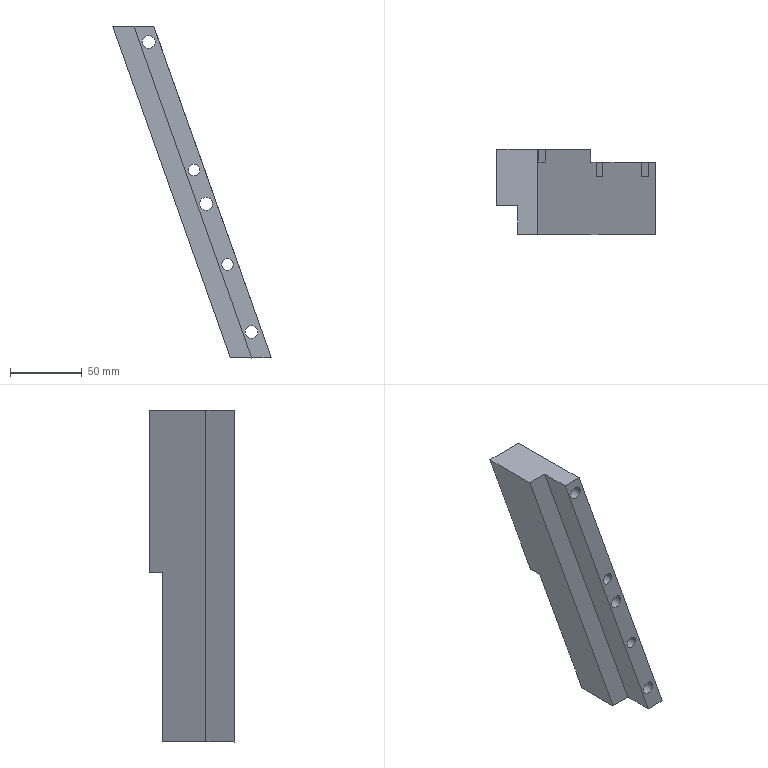Part | STEP file | SLIDE1-PLATE_id550_x_t | 1 solid | 27 faces | box 110.798 x 59.5 x 232 mm | volume 275836 mm3 | plane 19 | cylinder 8 | commonest cylinder face diameters 9 x3 14 x3 8 x2
STEP:
#1=CARTESIAN_POINT('',(86.433,-9.5,-60.698));
#2=VERTEX_POINT('',#1);
#3=CARTESIAN_POINT('',(81.759,-9.5,-47.502));
#4=VERTEX_POINT('',#3);
#5=CARTESIAN_POINT('',(84.096,-9.5,-54.1));
#6=DIRECTION('',(0.,1.,0.));
#7=DIRECTION('',(0.,0.,1.));
#8=AXIS2_PLACEMENT_3D('',#5,#6,#7);
#9=CIRCLE('',#8,7.);
#10=EDGE_CURVE('',#2,#4,#9,.T.);
#11=ORIENTED_EDGE('',*,*,#10,.F.);
#12=CARTESIAN_POINT('',(86.433,-0.5,-60.698));
#13=VERTEX_POINT('',#12);
#14=CARTESIAN_POINT('',(86.433,-0.5,-60.698));
#15=DIRECTION('',(0.,1.,0.));
#16=VECTOR('',#15,1.);
#17=LINE('',#14,#16);
#18=EDGE_CURVE('',#2,#13,#17,.T.);
#19=ORIENTED_EDGE('',*,*,#18,.T.);
#20=CARTESIAN_POINT('',(81.759,-0.5,-47.502));
#21=VERTEX_POINT('',#20);
#22=CARTESIAN_POINT('',(84.096,-0.5,-54.1));
#23=DIRECTION('',(0.,-1.,0.));
#24=DIRECTION('',(0.,0.,1.));
#25=AXIS2_PLACEMENT_3D('',#22,#23,#24);
#26=CIRCLE('',#25,7.);
#27=EDGE_CURVE('',#21,#13,#26,.T.);
#28=ORIENTED_EDGE('',*,*,#27,.F.);
#29=CARTESIAN_POINT('',(81.759,-0.5,-47.502));
#30=DIRECTION('',(0.,-1.,0.));
#31=VECTOR('',#30,1.);
#32=LINE('',#29,#31);
#33=EDGE_CURVE('',#21,#4,#32,.T.);
#34=ORIENTED_EDGE('',*,*,#33,.T.);
#35=EDGE_LOOP('',(#11,#19,#28,#34));
#36=FACE_OUTER_BOUND('',#35,.T.);
#37=CARTESIAN_POINT('',(84.096,-0.5,-54.1));
#38=DIRECTION('',(0.,1.,0.));
#39=DIRECTION('',(0.,0.,1.));
#40=AXIS2_PLACEMENT_3D('',#37,#38,#39);
#41=CYLINDRICAL_SURFACE('',#40,7.);
#42=ADVANCED_FACE('',(#36),#41,.F.);
#43=CARTESIAN_POINT('',(84.096,-60.,-49.6));
#44=VERTEX_POINT('',#43);
#45=CARTESIAN_POINT('',(84.096,-60.,-54.1));
#46=DIRECTION('',(0.,1.,0.));
#47=DIRECTION('',(0.,0.,1.));
#48=AXIS2_PLACEMENT_3D('',#45,#46,#47);
#49=CIRCLE('',#48,4.5);
#50=EDGE_CURVE('',#44,#44,#49,.T.);
#51=ORIENTED_EDGE('',*,*,#50,.F.);
#52=EDGE_LOOP('',(#51));
#53=FACE_BOUND('',#52,.T.);
#54=CARTESIAN_POINT('',(84.096,-9.5,-49.6));
#55=VERTEX_POINT('',#54);
#56=CARTESIAN_POINT('',(84.096,-9.5,-54.1));
#57=DIRECTION('',(0.,-1.,0.));
#58=DIRECTION('',(0.,0.,1.));
#59=AXIS2_PLACEMENT_3D('',#56,#57,#58);
#60=CIRCLE('',#59,4.5);
#61=EDGE_CURVE('',#55,#55,#60,.T.);
#62=ORIENTED_EDGE('',*,*,#61,.F.);
#63=EDGE_LOOP('',(#62));
#64=FACE_BOUND('',#63,.T.);
#65=CARTESIAN_POINT('',(84.096,-0.5,-54.1));
#66=DIRECTION('',(0.,1.,0.));
#67=DIRECTION('',(0.,0.,1.));
#68=AXIS2_PLACEMENT_3D('',#65,#66,#67);
#69=CYLINDRICAL_SURFACE('',#68,4.5);
#70=ADVANCED_FACE('',(#53,#64),#69,.F.);
#71=CARTESIAN_POINT('',(115.807,-60.,-139.65));
#72=VERTEX_POINT('',#71);
#73=CARTESIAN_POINT('',(115.807,-60.,-143.65));
#74=DIRECTION('',(0.,1.,0.));
#75=DIRECTION('',(0.,0.,1.));
#76=AXIS2_PLACEMENT_3D('',#73,#74,#75);
#77=CIRCLE('',#76,4.);
#78=EDGE_CURVE('',#72,#72,#77,.T.);
#79=ORIENTED_EDGE('',*,*,#78,.F.);
#80=EDGE_LOOP('',(#79));
#81=FACE_BOUND('',#80,.T.);
#82=CARTESIAN_POINT('',(115.807,-0.5,-139.65));
#83=VERTEX_POINT('',#82);
#84=CARTESIAN_POINT('',(115.807,-0.5,-143.65));
#85=DIRECTION('',(0.,-1.,0.));
#86=DIRECTION('',(0.,0.,1.));
#87=AXIS2_PLACEMENT_3D('',#84,#85,#86);
#88=CIRCLE('',#87,4.);
#89=EDGE_CURVE('',#83,#83,#88,.T.);
#90=ORIENTED_EDGE('',*,*,#89,.F.);
#91=EDGE_LOOP('',(#90));
#92=FACE_BOUND('',#91,.T.);
#93=CARTESIAN_POINT('',(115.807,-0.5,-143.65));
#94=DIRECTION('',(0.,1.,0.));
#95=DIRECTION('',(0.,0.,1.));
#96=AXIS2_PLACEMENT_3D('',#93,#94,#95);
#97=CYLINDRICAL_SURFACE('',#96,4.);
#98=ADVANCED_FACE('',(#81,#92),#97,.F.);
#99=CARTESIAN_POINT('',(124.15,-60.,-162.71));
#100=VERTEX_POINT('',#99);
#101=CARTESIAN_POINT('',(124.15,-60.,-167.21));
#102=DIRECTION('',(0.,1.,0.));
#103=DIRECTION('',(0.,0.,1.));
#104=AXIS2_PLACEMENT_3D('',#101,#102,#103);
#105=CIRCLE('',#104,4.5);
#106=EDGE_CURVE('',#100,#100,#105,.T.);
#107=ORIENTED_EDGE('',*,*,#106,.F.);
#108=EDGE_LOOP('',(#107));
#109=FACE_BOUND('',#108,.T.);
#110=CARTESIAN_POINT('',(124.15,-19.5,-162.71));
#111=VERTEX_POINT('',#110);
#112=CARTESIAN_POINT('',(124.15,-19.5,-167.21));
#113=DIRECTION('',(0.,-1.,0.));
#114=DIRECTION('',(0.,0.,1.));
#115=AXIS2_PLACEMENT_3D('',#112,#113,#114);
#116=CIRCLE('',#115,4.5);
#117=EDGE_CURVE('',#111,#111,#116,.T.);
#118=ORIENTED_EDGE('',*,*,#117,.F.);
#119=EDGE_LOOP('',(#118));
#120=FACE_BOUND('',#119,.T.);
#121=CARTESIAN_POINT('',(124.15,-0.5,-167.21));
#122=DIRECTION('',(0.,1.,0.));
#123=DIRECTION('',(0.,0.,1.));
#124=AXIS2_PLACEMENT_3D('',#121,#122,#123);
#125=CYLINDRICAL_SURFACE('',#124,4.5);
#126=ADVANCED_FACE('',(#109,#120),#125,.F.);
#127=CARTESIAN_POINT('',(155.862,-60.,-252.26));
#128=VERTEX_POINT('',#127);
#129=CARTESIAN_POINT('',(155.862,-60.,-256.76));
#130=DIRECTION('',(0.,1.,0.));
#131=DIRECTION('',(0.,0.,1.));
#132=AXIS2_PLACEMENT_3D('',#129,#130,#131);
#133=CIRCLE('',#132,4.5);
#134=EDGE_CURVE('',#128,#128,#133,.T.);
#135=ORIENTED_EDGE('',*,*,#134,.F.);
#136=EDGE_LOOP('',(#135));
#137=FACE_BOUND('',#136,.T.);
#138=CARTESIAN_POINT('',(155.862,-19.5,-252.26));
#139=VERTEX_POINT('',#138);
#140=CARTESIAN_POINT('',(155.862,-19.5,-256.76));
#141=DIRECTION('',(0.,-1.,0.));
#142=DIRECTION('',(0.,0.,1.));
#143=AXIS2_PLACEMENT_3D('',#140,#141,#142);
#144=CIRCLE('',#143,4.5);
#145=EDGE_CURVE('',#139,#139,#144,.T.);
#146=ORIENTED_EDGE('',*,*,#145,.F.);
#147=EDGE_LOOP('',(#146));
#148=FACE_BOUND('',#147,.T.);
#149=CARTESIAN_POINT('',(155.862,-0.5,-256.76));
#150=DIRECTION('',(0.,1.,0.));
#151=DIRECTION('',(0.,0.,1.));
#152=AXIS2_PLACEMENT_3D('',#149,#150,#151);
#153=CYLINDRICAL_SURFACE('',#152,4.5);
#154=ADVANCED_FACE('',(#137,#148),#153,.F.);
#155=CARTESIAN_POINT('',(155.956,-40.,-275.));
#156=VERTEX_POINT('',#155);
#157=CARTESIAN_POINT('',(73.8,-40.,-43.));
#158=VERTEX_POINT('',#157);
#159=CARTESIAN_POINT('',(63.323,-40.,-13.414));
#160=DIRECTION('',(-0.3338,0.,0.9426));
#161=VECTOR('',#160,1.);
#162=LINE('',#159,#161);
#163=EDGE_CURVE('',#156,#158,#162,.T.);
#164=ORIENTED_EDGE('',*,*,#163,.T.);
#165=CARTESIAN_POINT('',(58.948,-40.,-43.));
#166=VERTEX_POINT('',#165);
#167=CARTESIAN_POINT('',(83.348,-40.,-43.));
#168=DIRECTION('',(-1.,0.,0.));
#169=VECTOR('',#168,1.);
#170=LINE('',#167,#169);
#171=EDGE_CURVE('',#158,#166,#170,.T.);
#172=ORIENTED_EDGE('',*,*,#171,.T.);
#173=CARTESIAN_POINT('',(141.104,-40.,-275.));
#174=VERTEX_POINT('',#173);
#175=CARTESIAN_POINT('',(50.126,-40.,-18.087));
#176=DIRECTION('',(-0.3338,0.,0.9426));
#177=VECTOR('',#176,1.);
#178=LINE('',#175,#177);
#179=EDGE_CURVE('',#174,#166,#178,.T.);
#180=ORIENTED_EDGE('',*,*,#179,.F.);
#181=CARTESIAN_POINT('',(141.104,-40.,-275.));
#182=DIRECTION('',(1.,0.,0.));
#183=VECTOR('',#182,1.);
#184=LINE('',#181,#183);
#185=EDGE_CURVE('',#174,#156,#184,.T.);
#186=ORIENTED_EDGE('',*,*,#185,.T.);
#187=EDGE_LOOP('',(#164,#172,#180,#186));
#188=FACE_OUTER_BOUND('',#187,.T.);
#189=CARTESIAN_POINT('',(63.323,-40.,-13.414));
#190=DIRECTION('',(0.,1.,0.));
#191=DIRECTION('',(0.,0.,1.));
#192=AXIS2_PLACEMENT_3D('',#189,#190,#191);
#193=PLANE('',#192);
#194=ADVANCED_FACE('',(#188),#193,.F.);
#195=ORIENTED_EDGE('',*,*,#163,.F.);
#196=CARTESIAN_POINT('',(155.956,-60.,-275.));
#197=VERTEX_POINT('',#196);
#198=CARTESIAN_POINT('',(155.956,-0.5,-275.));
#199=DIRECTION('',(0.,-1.,0.));
#200=VECTOR('',#199,1.);
#201=LINE('',#198,#200);
#202=EDGE_CURVE('',#156,#197,#201,.T.);
#203=ORIENTED_EDGE('',*,*,#202,.T.);
#204=CARTESIAN_POINT('',(73.8,-60.,-43.));
#205=VERTEX_POINT('',#204);
#206=CARTESIAN_POINT('',(73.8,-60.,-43.));
#207=DIRECTION('',(0.3338,0.,-0.9426));
#208=VECTOR('',#207,1.);
#209=LINE('',#206,#208);
#210=EDGE_CURVE('',#205,#197,#209,.T.);
#211=ORIENTED_EDGE('',*,*,#210,.F.);
#212=CARTESIAN_POINT('',(73.8,-0.5,-43.));
#213=DIRECTION('',(0.,1.,0.));
#214=VECTOR('',#213,1.);
#215=LINE('',#212,#214);
#216=EDGE_CURVE('',#205,#158,#215,.T.);
#217=ORIENTED_EDGE('',*,*,#216,.T.);
#218=EDGE_LOOP('',(#195,#203,#211,#217));
#219=FACE_OUTER_BOUND('',#218,.T.);
#220=CARTESIAN_POINT('',(63.323,-60.,-13.414));
#221=DIRECTION('',(0.9426,0.,0.3338));
#222=DIRECTION('',(0.3338,0.,-0.9426));
#223=AXIS2_PLACEMENT_3D('',#220,#221,#222);
#224=PLANE('',#223);
#225=ADVANCED_FACE('',(#219),#224,.F.);
#226=CARTESIAN_POINT('',(126.487,-19.5,-173.808));
#227=VERTEX_POINT('',#226);
#228=CARTESIAN_POINT('',(121.814,-19.5,-160.612));
#229=VERTEX_POINT('',#228);
#230=CARTESIAN_POINT('',(124.15,-19.5,-167.21));
#231=DIRECTION('',(0.,1.,0.));
#232=DIRECTION('',(0.,0.,1.));
#233=AXIS2_PLACEMENT_3D('',#230,#231,#232);
#234=CIRCLE('',#233,7.);
#235=EDGE_CURVE('',#227,#229,#234,.T.);
#236=ORIENTED_EDGE('',*,*,#235,.F.);
#237=CARTESIAN_POINT('',(126.487,-9.5,-173.808));
#238=VERTEX_POINT('',#237);
#239=CARTESIAN_POINT('',(126.487,-0.5,-173.808));
#240=DIRECTION('',(0.,1.,0.));
#241=VECTOR('',#240,1.);
#242=LINE('',#239,#241);
#243=EDGE_CURVE('',#227,#238,#242,.T.);
#244=ORIENTED_EDGE('',*,*,#243,.T.);
#245=CARTESIAN_POINT('',(121.814,-9.5,-160.612));
#246=VERTEX_POINT('',#245);
#247=CARTESIAN_POINT('',(124.15,-9.5,-167.21));
#248=DIRECTION('',(0.,-1.,0.));
#249=DIRECTION('',(0.,0.,1.));
#250=AXIS2_PLACEMENT_3D('',#247,#248,#249);
#251=CIRCLE('',#250,7.);
#252=EDGE_CURVE('',#246,#238,#251,.T.);
#253=ORIENTED_EDGE('',*,*,#252,.F.);
#254=CARTESIAN_POINT('',(121.814,-0.5,-160.612));
#255=DIRECTION('',(0.,-1.,0.));
#256=VECTOR('',#255,1.);
#257=LINE('',#254,#256);
#258=EDGE_CURVE('',#246,#229,#257,.T.);
#259=ORIENTED_EDGE('',*,*,#258,.T.);
#260=EDGE_LOOP('',(#236,#244,#253,#259));
#261=FACE_OUTER_BOUND('',#260,.T.);
#262=CARTESIAN_POINT('',(124.15,-0.5,-167.21));
#263=DIRECTION('',(0.,1.,0.));
#264=DIRECTION('',(0.,0.,1.));
#265=AXIS2_PLACEMENT_3D('',#262,#263,#264);
#266=CYLINDRICAL_SURFACE('',#265,7.);
#267=ADVANCED_FACE('',(#261),#266,.F.);
#268=CARTESIAN_POINT('',(158.198,-19.5,-263.358));
#269=VERTEX_POINT('',#268);
#270=CARTESIAN_POINT('',(153.525,-19.5,-250.162));
#271=VERTEX_POINT('',#270);
#272=CARTESIAN_POINT('',(155.862,-19.5,-256.76));
#273=DIRECTION('',(0.,1.,0.));
#274=DIRECTION('',(0.,0.,1.));
#275=AXIS2_PLACEMENT_3D('',#272,#273,#274);
#276=CIRCLE('',#275,7.);
#277=EDGE_CURVE('',#269,#271,#276,.T.);
#278=ORIENTED_EDGE('',*,*,#277,.F.);
#279=CARTESIAN_POINT('',(158.198,-9.5,-263.358));
#280=VERTEX_POINT('',#279);
#281=CARTESIAN_POINT('',(158.198,-0.5,-263.358));
#282=DIRECTION('',(0.,1.,0.));
#283=VECTOR('',#282,1.);
#284=LINE('',#281,#283);
#285=EDGE_CURVE('',#269,#280,#284,.T.);
#286=ORIENTED_EDGE('',*,*,#285,.T.);
#287=CARTESIAN_POINT('',(153.525,-9.5,-250.162));
#288=VERTEX_POINT('',#287);
#289=CARTESIAN_POINT('',(155.862,-9.5,-256.76));
#290=DIRECTION('',(0.,-1.,0.));
#291=DIRECTION('',(0.,0.,1.));
#292=AXIS2_PLACEMENT_3D('',#289,#290,#291);
#293=CIRCLE('',#292,7.);
#294=EDGE_CURVE('',#288,#280,#293,.T.);
#295=ORIENTED_EDGE('',*,*,#294,.F.);
#296=CARTESIAN_POINT('',(153.525,-0.5,-250.162));
#297=DIRECTION('',(0.,-1.,0.));
#298=VECTOR('',#297,1.);
#299=LINE('',#296,#298);
#300=EDGE_CURVE('',#288,#271,#299,.T.);
#301=ORIENTED_EDGE('',*,*,#300,.T.);
#302=EDGE_LOOP('',(#278,#286,#295,#301));
#303=FACE_OUTER_BOUND('',#302,.T.);
#304=CARTESIAN_POINT('',(155.862,-0.5,-256.76));
#305=DIRECTION('',(0.,1.,0.));
#306=DIRECTION('',(0.,0.,1.));
#307=AXIS2_PLACEMENT_3D('',#304,#305,#306);
#308=CYLINDRICAL_SURFACE('',#307,7.);
#309=ADVANCED_FACE('',(#303),#308,.F.);
#310=CARTESIAN_POINT('',(99.196,-0.5,-156.656));
#311=VERTEX_POINT('',#310);
#312=CARTESIAN_POINT('',(99.196,-9.5,-156.656));
#313=VERTEX_POINT('',#312);
#314=CARTESIAN_POINT('',(99.196,-0.5,-156.656));
#315=DIRECTION('',(0.,-1.,0.));
#316=VECTOR('',#315,1.);
#317=LINE('',#314,#316);
#318=EDGE_CURVE('',#311,#313,#317,.T.);
#319=ORIENTED_EDGE('',*,*,#318,.T.);
#320=CARTESIAN_POINT('',(141.104,-9.5,-275.));
#321=VERTEX_POINT('',#320);
#322=CARTESIAN_POINT('',(141.104,-9.5,-275.));
#323=DIRECTION('',(-0.3338,0.,0.9426));
#324=VECTOR('',#323,1.);
#325=LINE('',#322,#324);
#326=EDGE_CURVE('',#321,#313,#325,.T.);
#327=ORIENTED_EDGE('',*,*,#326,.F.);
#328=CARTESIAN_POINT('',(141.104,-0.5,-275.));
#329=DIRECTION('',(0.,-1.,0.));
#330=VECTOR('',#329,1.);
#331=LINE('',#328,#330);
#332=EDGE_CURVE('',#321,#174,#331,.T.);
#333=ORIENTED_EDGE('',*,*,#332,.T.);
#334=ORIENTED_EDGE('',*,*,#179,.T.);
#335=CARTESIAN_POINT('',(58.948,-0.5,-43.));
#336=VERTEX_POINT('',#335);
#337=CARTESIAN_POINT('',(58.948,-0.5,-43.));
#338=DIRECTION('',(0.,1.,0.));
#339=VECTOR('',#338,1.);
#340=LINE('',#337,#339);
#341=EDGE_CURVE('',#166,#336,#340,.T.);
#342=ORIENTED_EDGE('',*,*,#341,.T.);
#343=CARTESIAN_POINT('',(99.196,-0.5,-156.656));
#344=DIRECTION('',(-0.3338,0.,0.9426));
#345=VECTOR('',#344,1.);
#346=LINE('',#343,#345);
#347=EDGE_CURVE('',#311,#336,#346,.T.);
#348=ORIENTED_EDGE('',*,*,#347,.F.);
#349=EDGE_LOOP('',(#319,#327,#333,#334,#342,#348));
#350=FACE_OUTER_BOUND('',#349,.T.);
#351=CARTESIAN_POINT('',(50.126,-50.,-18.087));
#352=DIRECTION('',(-0.9426,0.,-0.3338));
#353=DIRECTION('',(-0.3338,0.,0.9426));
#354=AXIS2_PLACEMENT_3D('',#351,#352,#353);
#355=PLANE('',#354);
#356=ADVANCED_FACE('',(#350),#355,.T.);
#357=CARTESIAN_POINT('',(139.172,-60.,-205.63));
#358=VERTEX_POINT('',#357);
#359=CARTESIAN_POINT('',(139.172,-60.,-209.63));
#360=DIRECTION('',(0.,1.,0.));
#361=DIRECTION('',(0.,0.,1.));
#362=AXIS2_PLACEMENT_3D('',#359,#360,#361);
#363=CIRCLE('',#362,4.);
#364=EDGE_CURVE('',#358,#358,#363,.T.);
#365=ORIENTED_EDGE('',*,*,#364,.F.);
#366=EDGE_LOOP('',(#365));
#367=FACE_BOUND('',#366,.T.);
#368=CARTESIAN_POINT('',(139.172,-9.5,-205.63));
#369=VERTEX_POINT('',#368);
#370=CARTESIAN_POINT('',(139.172,-9.5,-209.63));
#371=DIRECTION('',(0.,-1.,0.));
#372=DIRECTION('',(0.,0.,1.));
#373=AXIS2_PLACEMENT_3D('',#370,#371,#372);
#374=CIRCLE('',#373,4.);
#375=EDGE_CURVE('',#369,#369,#374,.T.);
#376=ORIENTED_EDGE('',*,*,#375,.F.);
#377=EDGE_LOOP('',(#376));
#378=FACE_BOUND('',#377,.T.);
#379=CARTESIAN_POINT('',(139.172,-0.5,-209.63));
#380=DIRECTION('',(0.,1.,0.));
#381=DIRECTION('',(0.,0.,1.));
#382=AXIS2_PLACEMENT_3D('',#379,#380,#381);
#383=CYLINDRICAL_SURFACE('',#382,4.);
#384=ADVANCED_FACE('',(#367,#378),#383,.F.);
#385=CARTESIAN_POINT('',(164.797,-19.5,-261.022));
#386=VERTEX_POINT('',#385);
#387=CARTESIAN_POINT('',(164.797,-19.5,-261.022));
#388=DIRECTION('',(-0.9426,0.,-0.3338));
#389=VECTOR('',#388,1.);
#390=LINE('',#387,#389);
#391=EDGE_CURVE('',#386,#269,#390,.T.);
#392=ORIENTED_EDGE('',*,*,#391,.F.);
#393=CARTESIAN_POINT('',(164.797,-9.5,-261.022));
#394=VERTEX_POINT('',#393);
#395=CARTESIAN_POINT('',(164.797,-0.5,-261.022));
#396=DIRECTION('',(0.,-1.,0.));
#397=VECTOR('',#396,1.);
#398=LINE('',#395,#397);
#399=EDGE_CURVE('',#394,#386,#398,.T.);
#400=ORIENTED_EDGE('',*,*,#399,.F.);
#401=CARTESIAN_POINT('',(158.198,-9.5,-263.358));
#402=DIRECTION('',(0.9426,0.,0.3338));
#403=VECTOR('',#402,1.);
#404=LINE('',#401,#403);
#405=EDGE_CURVE('',#280,#394,#404,.T.);
#406=ORIENTED_EDGE('',*,*,#405,.F.);
#407=ORIENTED_EDGE('',*,*,#285,.F.);
#408=EDGE_LOOP('',(#392,#400,#406,#407));
#409=FACE_OUTER_BOUND('',#408,.T.);
#410=CARTESIAN_POINT('',(168.006,-0.5,-259.886));
#411=DIRECTION('',(0.3338,0.,-0.9426));
#412=DIRECTION('',(-0.9426,0.,-0.3338));
#413=AXIS2_PLACEMENT_3D('',#410,#411,#412);
#414=PLANE('',#413);
#415=ADVANCED_FACE('',(#409),#414,.F.);
#416=ORIENTED_EDGE('',*,*,#145,.T.);
#417=EDGE_LOOP('',(#416));
#418=FACE_BOUND('',#417,.T.);
#419=CARTESIAN_POINT('',(160.123,-19.5,-247.825));
#420=VERTEX_POINT('',#419);
#421=CARTESIAN_POINT('',(153.525,-19.5,-250.162));
#422=DIRECTION('',(0.9426,0.,0.3338));
#423=VECTOR('',#422,1.);
#424=LINE('',#421,#423);
#425=EDGE_CURVE('',#271,#420,#424,.T.);
#426=ORIENTED_EDGE('',*,*,#425,.T.);
#427=CARTESIAN_POINT('',(169.747,-19.5,-275.));
#428=DIRECTION('',(-0.3338,0.,0.9426));
#429=VECTOR('',#428,1.);
#430=LINE('',#427,#429);
#431=EDGE_CURVE('',#386,#420,#430,.T.);
#432=ORIENTED_EDGE('',*,*,#431,.F.);
#433=ORIENTED_EDGE('',*,*,#391,.T.);
#434=ORIENTED_EDGE('',*,*,#277,.T.);
#435=EDGE_LOOP('',(#426,#432,#433,#434));
#436=FACE_BOUND('',#435,.T.);
#437=CARTESIAN_POINT('',(11.277,-19.5,-31.845));
#438=DIRECTION('',(0.,1.,0.));
#439=DIRECTION('',(0.,0.,1.));
#440=AXIS2_PLACEMENT_3D('',#437,#438,#439);
#441=PLANE('',#440);
#442=ADVANCED_FACE('',(#418,#436),#441,.T.);
#443=ORIENTED_EDGE('',*,*,#425,.F.);
#444=ORIENTED_EDGE('',*,*,#300,.F.);
#445=CARTESIAN_POINT('',(160.123,-9.5,-247.825));
#446=VERTEX_POINT('',#445);
#447=CARTESIAN_POINT('',(160.123,-9.5,-247.825));
#448=DIRECTION('',(-0.9426,0.,-0.3338));
#449=VECTOR('',#448,1.);
#450=LINE('',#447,#449);
#451=EDGE_CURVE('',#446,#288,#450,.T.);
#452=ORIENTED_EDGE('',*,*,#451,.F.);
#453=CARTESIAN_POINT('',(160.123,-0.5,-247.825));
#454=DIRECTION('',(0.,1.,0.));
#455=VECTOR('',#454,1.);
#456=LINE('',#453,#455);
#457=EDGE_CURVE('',#420,#446,#456,.T.);
#458=ORIENTED_EDGE('',*,*,#457,.F.);
#459=EDGE_LOOP('',(#443,#444,#452,#458));
#460=FACE_OUTER_BOUND('',#459,.T.);
#461=CARTESIAN_POINT('',(153.525,-0.5,-250.162));
#462=DIRECTION('',(-0.3338,0.,0.9426));
#463=DIRECTION('',(0.9426,0.,0.3338));
#464=AXIS2_PLACEMENT_3D('',#461,#462,#463);
#465=PLANE('',#464);
#466=ADVANCED_FACE('',(#460),#465,.F.);
#467=CARTESIAN_POINT('',(133.085,-19.5,-171.472));
#468=VERTEX_POINT('',#467);
#469=CARTESIAN_POINT('',(133.085,-19.5,-171.472));
#470=DIRECTION('',(-0.9426,0.,-0.3338));
#471=VECTOR('',#470,1.);
#472=LINE('',#469,#471);
#473=EDGE_CURVE('',#468,#227,#472,.T.);
#474=ORIENTED_EDGE('',*,*,#473,.F.);
#475=CARTESIAN_POINT('',(133.085,-9.5,-171.472));
#476=VERTEX_POINT('',#475);
#477=CARTESIAN_POINT('',(133.085,-0.5,-171.472));
#478=DIRECTION('',(0.,-1.,0.));
#479=VECTOR('',#478,1.);
#480=LINE('',#477,#479);
#481=EDGE_CURVE('',#476,#468,#480,.T.);
#482=ORIENTED_EDGE('',*,*,#481,.F.);
#483=CARTESIAN_POINT('',(126.487,-9.5,-173.808));
#484=DIRECTION('',(0.9426,0.,0.3338));
#485=VECTOR('',#484,1.);
#486=LINE('',#483,#485);
#487=EDGE_CURVE('',#238,#476,#486,.T.);
#488=ORIENTED_EDGE('',*,*,#487,.F.);
#489=ORIENTED_EDGE('',*,*,#243,.F.);
#490=EDGE_LOOP('',(#474,#482,#488,#489));
#491=FACE_OUTER_BOUND('',#490,.T.);
#492=CARTESIAN_POINT('',(136.294,-0.5,-170.336));
#493=DIRECTION('',(0.3338,0.,-0.9426));
#494=DIRECTION('',(-0.9426,0.,-0.3338));
#495=AXIS2_PLACEMENT_3D('',#492,#493,#494);
#496=PLANE('',#495);
#497=ADVANCED_FACE('',(#491),#496,.F.);
#498=ORIENTED_EDGE('',*,*,#117,.T.);
#499=EDGE_LOOP('',(#498));
#500=FACE_BOUND('',#499,.T.);
#501=CARTESIAN_POINT('',(128.412,-19.5,-158.275));
#502=VERTEX_POINT('',#501);
#503=CARTESIAN_POINT('',(121.814,-19.5,-160.612));
#504=DIRECTION('',(0.9426,0.,0.3338));
#505=VECTOR('',#504,1.);
#506=LINE('',#503,#505);
#507=EDGE_CURVE('',#229,#502,#506,.T.);
#508=ORIENTED_EDGE('',*,*,#507,.T.);
#509=CARTESIAN_POINT('',(169.747,-19.5,-275.));
#510=DIRECTION('',(-0.3338,0.,0.9426));
#511=VECTOR('',#510,1.);
#512=LINE('',#509,#511);
#513=EDGE_CURVE('',#468,#502,#512,.T.);
#514=ORIENTED_EDGE('',*,*,#513,.F.);
#515=ORIENTED_EDGE('',*,*,#473,.T.);
#516=ORIENTED_EDGE('',*,*,#235,.T.);
#517=EDGE_LOOP('',(#508,#514,#515,#516));
#518=FACE_BOUND('',#517,.T.);
#519=CARTESIAN_POINT('',(11.277,-19.5,-31.845));
#520=DIRECTION('',(0.,1.,0.));
#521=DIRECTION('',(0.,0.,1.));
#522=AXIS2_PLACEMENT_3D('',#519,#520,#521);
#523=PLANE('',#522);
#524=ADVANCED_FACE('',(#500,#518),#523,.T.);
#525=ORIENTED_EDGE('',*,*,#507,.F.);
#526=ORIENTED_EDGE('',*,*,#258,.F.);
#527=CARTESIAN_POINT('',(128.412,-9.5,-158.275));
#528=VERTEX_POINT('',#527);
#529=CARTESIAN_POINT('',(128.412,-9.5,-158.275));
#530=DIRECTION('',(-0.9426,0.,-0.3338));
#531=VECTOR('',#530,1.);
#532=LINE('',#529,#531);
#533=EDGE_CURVE('',#528,#246,#532,.T.);
#534=ORIENTED_EDGE('',*,*,#533,.F.);
#535=CARTESIAN_POINT('',(128.412,-0.5,-158.275));
#536=DIRECTION('',(0.,1.,0.));
#537=VECTOR('',#536,1.);
#538=LINE('',#535,#537);
#539=EDGE_CURVE('',#502,#528,#538,.T.);
#540=ORIENTED_EDGE('',*,*,#539,.F.);
#541=EDGE_LOOP('',(#525,#526,#534,#540));
#542=FACE_OUTER_BOUND('',#541,.T.);
#543=CARTESIAN_POINT('',(121.814,-0.5,-160.612));
#544=DIRECTION('',(-0.3338,0.,0.9426));
#545=DIRECTION('',(0.9426,0.,0.3338));
#546=AXIS2_PLACEMENT_3D('',#543,#544,#545);
#547=PLANE('',#546);
#548=ADVANCED_FACE('',(#542),#547,.F.);
#549=CARTESIAN_POINT('',(124.647,-9.5,-147.643));
#550=VERTEX_POINT('',#549);
#551=CARTESIAN_POINT('',(99.196,-9.5,-156.656));
#552=DIRECTION('',(0.9426,0.,0.3338));
#553=VECTOR('',#552,1.);
#554=LINE('',#551,#553);
#555=EDGE_CURVE('',#313,#550,#554,.T.);
#556=ORIENTED_EDGE('',*,*,#555,.F.);
#557=ORIENTED_EDGE('',*,*,#318,.F.);
#558=CARTESIAN_POINT('',(124.647,-0.5,-147.643));
#559=VERTEX_POINT('',#558);
#560=CARTESIAN_POINT('',(124.647,-0.5,-147.643));
#561=DIRECTION('',(-0.9426,0.,-0.3338));
#562=VECTOR('',#561,1.);
#563=LINE('',#560,#562);
#564=EDGE_CURVE('',#559,#311,#563,.T.);
#565=ORIENTED_EDGE('',*,*,#564,.F.);
#566=CARTESIAN_POINT('',(124.647,-0.5,-147.643));
#567=DIRECTION('',(0.,1.,0.));
#568=VECTOR('',#567,1.);
#569=LINE('',#566,#568);
#570=EDGE_CURVE('',#550,#559,#569,.T.);
#571=ORIENTED_EDGE('',*,*,#570,.F.);
#572=EDGE_LOOP('',(#556,#557,#565,#571));
#573=FACE_OUTER_BOUND('',#572,.T.);
#574=CARTESIAN_POINT('',(-26.175,-0.5,-201.052));
#575=DIRECTION('',(-0.3338,0.,0.9426));
#576=DIRECTION('',(0.9426,0.,0.3338));
#577=AXIS2_PLACEMENT_3D('',#574,#575,#576);
#578=PLANE('',#577);
#579=ADVANCED_FACE('',(#573),#578,.F.);
#580=CARTESIAN_POINT('',(93.031,-9.5,-58.362));
#581=VERTEX_POINT('',#580);
#582=CARTESIAN_POINT('',(93.031,-9.5,-58.362));
#583=DIRECTION('',(-0.9426,0.,-0.3338));
#584=VECTOR('',#583,1.);
#585=LINE('',#582,#584);
#586=EDGE_CURVE('',#581,#2,#585,.T.);
#587=ORIENTED_EDGE('',*,*,#586,.F.);
#588=CARTESIAN_POINT('',(93.031,-0.5,-58.362));
#589=VERTEX_POINT('',#588);
#590=CARTESIAN_POINT('',(93.031,-0.5,-58.362));
#591=DIRECTION('',(0.,-1.,0.));
#592=VECTOR('',#591,1.);
#593=LINE('',#590,#592);
#594=EDGE_CURVE('',#589,#581,#593,.T.);
#595=ORIENTED_EDGE('',*,*,#594,.F.);
#596=CARTESIAN_POINT('',(86.433,-0.5,-60.698));
#597=DIRECTION('',(0.9426,0.,0.3338));
#598=VECTOR('',#597,1.);
#599=LINE('',#596,#598);
#600=EDGE_CURVE('',#13,#589,#599,.T.);
#601=ORIENTED_EDGE('',*,*,#600,.F.);
#602=ORIENTED_EDGE('',*,*,#18,.F.);
#603=EDGE_LOOP('',(#587,#595,#601,#602));
#604=FACE_OUTER_BOUND('',#603,.T.);
#605=CARTESIAN_POINT('',(96.24,-0.5,-57.226));
#606=DIRECTION('',(0.3338,0.,-0.9426));
#607=DIRECTION('',(-0.9426,0.,-0.3338));
#608=AXIS2_PLACEMENT_3D('',#605,#606,#607);
#609=PLANE('',#608);
#610=ADVANCED_FACE('',(#604),#609,.F.);
#611=ORIENTED_EDGE('',*,*,#61,.T.);
#612=EDGE_LOOP('',(#611));
#613=FACE_BOUND('',#612,.T.);
#614=CARTESIAN_POINT('',(88.358,-9.5,-45.165));
#615=VERTEX_POINT('',#614);
#616=CARTESIAN_POINT('',(81.759,-9.5,-47.502));
#617=DIRECTION('',(0.9426,0.,0.3338));
#618=VECTOR('',#617,1.);
#619=LINE('',#616,#618);
#620=EDGE_CURVE('',#4,#615,#619,.T.);
#621=ORIENTED_EDGE('',*,*,#620,.T.);
#622=CARTESIAN_POINT('',(169.747,-9.5,-275.));
#623=DIRECTION('',(-0.3338,0.,0.9426));
#624=VECTOR('',#623,1.);
#625=LINE('',#622,#624);
#626=EDGE_CURVE('',#581,#615,#625,.T.);
#627=ORIENTED_EDGE('',*,*,#626,.F.);
#628=ORIENTED_EDGE('',*,*,#586,.T.);
#629=ORIENTED_EDGE('',*,*,#10,.T.);
#630=EDGE_LOOP('',(#621,#627,#628,#629));
#631=FACE_BOUND('',#630,.T.);
#632=CARTESIAN_POINT('',(11.277,-9.5,-31.845));
#633=DIRECTION('',(0.,1.,0.));
#634=DIRECTION('',(0.,0.,1.));
#635=AXIS2_PLACEMENT_3D('',#632,#633,#634);
#636=PLANE('',#635);
#637=ADVANCED_FACE('',(#613,#631),#636,.T.);
#638=ORIENTED_EDGE('',*,*,#620,.F.);
#639=ORIENTED_EDGE('',*,*,#33,.F.);
#640=CARTESIAN_POINT('',(88.358,-0.5,-45.165));
#641=VERTEX_POINT('',#640);
#642=CARTESIAN_POINT('',(88.358,-0.5,-45.165));
#643=DIRECTION('',(-0.9426,0.,-0.3338));
#644=VECTOR('',#643,1.);
#645=LINE('',#642,#644);
#646=EDGE_CURVE('',#641,#21,#645,.T.);
#647=ORIENTED_EDGE('',*,*,#646,.F.);
#648=CARTESIAN_POINT('',(88.358,-0.5,-45.165));
#649=DIRECTION('',(0.,1.,0.));
#650=VECTOR('',#649,1.);
#651=LINE('',#648,#650);
#652=EDGE_CURVE('',#615,#641,#651,.T.);
#653=ORIENTED_EDGE('',*,*,#652,.F.);
#654=EDGE_LOOP('',(#638,#639,#647,#653));
#655=FACE_OUTER_BOUND('',#654,.T.);
#656=CARTESIAN_POINT('',(81.759,-0.5,-47.502));
#657=DIRECTION('',(-0.3338,0.,0.9426));
#658=DIRECTION('',(0.9426,0.,0.3338));
#659=AXIS2_PLACEMENT_3D('',#656,#657,#658);
#660=PLANE('',#659);
#661=ADVANCED_FACE('',(#655),#660,.F.);
#662=ORIENTED_EDGE('',*,*,#89,.T.);
#663=EDGE_LOOP('',(#662));
#664=FACE_BOUND('',#663,.T.);
#665=CARTESIAN_POINT('',(169.747,-0.5,-275.));
#666=DIRECTION('',(-0.3338,0.,0.9426));
#667=VECTOR('',#666,1.);
#668=LINE('',#665,#667);
#669=EDGE_CURVE('',#559,#589,#668,.T.);
#670=ORIENTED_EDGE('',*,*,#669,.F.);
#671=ORIENTED_EDGE('',*,*,#564,.T.);
#672=ORIENTED_EDGE('',*,*,#347,.T.);
#673=CARTESIAN_POINT('',(87.591,-0.5,-43.));
#674=VERTEX_POINT('',#673);
#675=CARTESIAN_POINT('',(83.348,-0.5,-43.));
#676=DIRECTION('',(1.,0.,0.));
#677=VECTOR('',#676,1.);
#678=LINE('',#675,#677);
#679=EDGE_CURVE('',#336,#674,#678,.T.);
#680=ORIENTED_EDGE('',*,*,#679,.T.);
#681=CARTESIAN_POINT('',(169.747,-0.5,-275.));
#682=DIRECTION('',(-0.3338,0.,0.9426));
#683=VECTOR('',#682,1.);
#684=LINE('',#681,#683);
#685=EDGE_CURVE('',#641,#674,#684,.T.);
#686=ORIENTED_EDGE('',*,*,#685,.F.);
#687=ORIENTED_EDGE('',*,*,#646,.T.);
#688=ORIENTED_EDGE('',*,*,#27,.T.);
#689=ORIENTED_EDGE('',*,*,#600,.T.);
#690=EDGE_LOOP('',(#670,#671,#672,#680,#686,#687,#688,#689));
#691=FACE_BOUND('',#690,.T.);
#692=CARTESIAN_POINT('',(-84.671,-0.5,-65.822));
#693=DIRECTION('',(0.,1.,0.));
#694=DIRECTION('',(0.,0.,1.));
#695=AXIS2_PLACEMENT_3D('',#692,#693,#694);
#696=PLANE('',#695);
#697=ADVANCED_FACE('',(#664,#691),#696,.T.);
#698=CARTESIAN_POINT('',(87.591,-60.,-43.));
#699=VERTEX_POINT('',#698);
#700=CARTESIAN_POINT('',(87.591,-0.5,-43.));
#701=DIRECTION('',(0.,-1.,0.));
#702=VECTOR('',#701,1.);
#703=LINE('',#700,#702);
#704=EDGE_CURVE('',#674,#699,#703,.T.);
#705=ORIENTED_EDGE('',*,*,#704,.F.);
#706=ORIENTED_EDGE('',*,*,#679,.F.);
#707=ORIENTED_EDGE('',*,*,#341,.F.);
#708=ORIENTED_EDGE('',*,*,#171,.F.);
#709=ORIENTED_EDGE('',*,*,#216,.F.);
#710=CARTESIAN_POINT('',(-70.532,-60.,-43.));
#711=DIRECTION('',(-1.,0.,0.));
#712=VECTOR('',#711,1.);
#713=LINE('',#710,#712);
#714=EDGE_CURVE('',#699,#205,#713,.T.);
#715=ORIENTED_EDGE('',*,*,#714,.F.);
#716=EDGE_LOOP('',(#705,#706,#707,#708,#709,#715));
#717=FACE_OUTER_BOUND('',#716,.T.);
#718=CARTESIAN_POINT('',(83.348,-0.5,-43.));
#719=DIRECTION('',(0.,0.,-1.));
#720=DIRECTION('',(-1.,0.,0.));
#721=AXIS2_PLACEMENT_3D('',#718,#719,#720);
#722=PLANE('',#721);
#723=ADVANCED_FACE('',(#717),#722,.F.);
#724=ORIENTED_EDGE('',*,*,#134,.T.);
#725=EDGE_LOOP('',(#724));
#726=FACE_BOUND('',#725,.T.);
#727=ORIENTED_EDGE('',*,*,#364,.T.);
#728=EDGE_LOOP('',(#727));
#729=FACE_BOUND('',#728,.T.);
#730=ORIENTED_EDGE('',*,*,#106,.T.);
#731=EDGE_LOOP('',(#730));
#732=FACE_BOUND('',#731,.T.);
#733=ORIENTED_EDGE('',*,*,#78,.T.);
#734=EDGE_LOOP('',(#733));
#735=FACE_BOUND('',#734,.T.);
#736=ORIENTED_EDGE('',*,*,#50,.T.);
#737=EDGE_LOOP('',(#736));
#738=FACE_BOUND('',#737,.T.);
#739=ORIENTED_EDGE('',*,*,#714,.T.);
#740=ORIENTED_EDGE('',*,*,#210,.T.);
#741=CARTESIAN_POINT('',(169.747,-60.,-275.));
#742=VERTEX_POINT('',#741);
#743=CARTESIAN_POINT('',(141.104,-60.,-275.));
#744=DIRECTION('',(1.,0.,0.));
#745=VECTOR('',#744,1.);
#746=LINE('',#743,#745);
#747=EDGE_CURVE('',#197,#742,#746,.T.);
#748=ORIENTED_EDGE('',*,*,#747,.T.);
#749=CARTESIAN_POINT('',(169.747,-60.,-275.));
#750=DIRECTION('',(0.3338,0.,-0.9426));
#751=VECTOR('',#750,1.);
#752=LINE('',#749,#751);
#753=EDGE_CURVE('',#699,#742,#752,.T.);
#754=ORIENTED_EDGE('',*,*,#753,.F.);
#755=EDGE_LOOP('',(#739,#740,#748,#754));
#756=FACE_BOUND('',#755,.T.);
#757=CARTESIAN_POINT('',(-70.532,-60.,-60.815));
#758=DIRECTION('',(0.,-1.,0.));
#759=DIRECTION('',(0.,0.,-1.));
#760=AXIS2_PLACEMENT_3D('',#757,#758,#759);
#761=PLANE('',#760);
#762=ADVANCED_FACE('',(#726,#729,#732,#735,#738,#756),#761,.T.);
#763=ORIENTED_EDGE('',*,*,#747,.F.);
#764=ORIENTED_EDGE('',*,*,#202,.F.);
#765=ORIENTED_EDGE('',*,*,#185,.F.);
#766=ORIENTED_EDGE('',*,*,#332,.F.);
#767=CARTESIAN_POINT('',(169.747,-9.5,-275.));
#768=VERTEX_POINT('',#767);
#769=CARTESIAN_POINT('',(11.277,-9.5,-275.));
#770=DIRECTION('',(-1.,0.,0.));
#771=VECTOR('',#770,1.);
#772=LINE('',#769,#771);
#773=EDGE_CURVE('',#768,#321,#772,.T.);
#774=ORIENTED_EDGE('',*,*,#773,.F.);
#775=CARTESIAN_POINT('',(169.747,-0.5,-275.));
#776=DIRECTION('',(0.,1.,0.));
#777=VECTOR('',#776,1.);
#778=LINE('',#775,#777);
#779=EDGE_CURVE('',#742,#768,#778,.T.);
#780=ORIENTED_EDGE('',*,*,#779,.F.);
#781=EDGE_LOOP('',(#763,#764,#765,#766,#774,#780));
#782=FACE_OUTER_BOUND('',#781,.T.);
#783=CARTESIAN_POINT('',(141.104,-0.5,-275.));
#784=DIRECTION('',(0.,0.,1.));
#785=DIRECTION('',(1.,0.,0.));
#786=AXIS2_PLACEMENT_3D('',#783,#784,#785);
#787=PLANE('',#786);
#788=ADVANCED_FACE('',(#782),#787,.F.);
#789=ORIENTED_EDGE('',*,*,#375,.T.);
#790=EDGE_LOOP('',(#789));
#791=FACE_BOUND('',#790,.T.);
#792=ORIENTED_EDGE('',*,*,#773,.T.);
#793=ORIENTED_EDGE('',*,*,#326,.T.);
#794=ORIENTED_EDGE('',*,*,#555,.T.);
#795=CARTESIAN_POINT('',(169.747,-9.5,-275.));
#796=DIRECTION('',(-0.3338,0.,0.9426));
#797=VECTOR('',#796,1.);
#798=LINE('',#795,#797);
#799=EDGE_CURVE('',#528,#550,#798,.T.);
#800=ORIENTED_EDGE('',*,*,#799,.F.);
#801=ORIENTED_EDGE('',*,*,#533,.T.);
#802=ORIENTED_EDGE('',*,*,#252,.T.);
#803=ORIENTED_EDGE('',*,*,#487,.T.);
#804=CARTESIAN_POINT('',(169.747,-9.5,-275.));
#805=DIRECTION('',(-0.3338,0.,0.9426));
#806=VECTOR('',#805,1.);
#807=LINE('',#804,#806);
#808=EDGE_CURVE('',#446,#476,#807,.T.);
#809=ORIENTED_EDGE('',*,*,#808,.F.);
#810=ORIENTED_EDGE('',*,*,#451,.T.);
#811=ORIENTED_EDGE('',*,*,#294,.T.);
#812=ORIENTED_EDGE('',*,*,#405,.T.);
#813=CARTESIAN_POINT('',(169.747,-9.5,-275.));
#814=DIRECTION('',(-0.3338,0.,0.9426));
#815=VECTOR('',#814,1.);
#816=LINE('',#813,#815);
#817=EDGE_CURVE('',#768,#394,#816,.T.);
#818=ORIENTED_EDGE('',*,*,#817,.F.);
#819=EDGE_LOOP('',(#792,#793,#794,#800,#801,#802,#803,#809,#810,#811,#812,#818));
#820=FACE_BOUND('',#819,.T.);
#821=CARTESIAN_POINT('',(11.277,-9.5,-31.845));
#822=DIRECTION('',(0.,1.,0.));
#823=DIRECTION('',(0.,0.,1.));
#824=AXIS2_PLACEMENT_3D('',#821,#822,#823);
#825=PLANE('',#824);
#826=ADVANCED_FACE('',(#791,#820),#825,.T.);
#827=ORIENTED_EDGE('',*,*,#779,.T.);
#828=ORIENTED_EDGE('',*,*,#817,.T.);
#829=ORIENTED_EDGE('',*,*,#399,.T.);
#830=ORIENTED_EDGE('',*,*,#431,.T.);
#831=ORIENTED_EDGE('',*,*,#457,.T.);
#832=ORIENTED_EDGE('',*,*,#808,.T.);
#833=ORIENTED_EDGE('',*,*,#481,.T.);
#834=ORIENTED_EDGE('',*,*,#513,.T.);
#835=ORIENTED_EDGE('',*,*,#539,.T.);
#836=ORIENTED_EDGE('',*,*,#799,.T.);
#837=ORIENTED_EDGE('',*,*,#570,.T.);
#838=ORIENTED_EDGE('',*,*,#669,.T.);
#839=ORIENTED_EDGE('',*,*,#594,.T.);
#840=ORIENTED_EDGE('',*,*,#626,.T.);
#841=ORIENTED_EDGE('',*,*,#652,.T.);
#842=ORIENTED_EDGE('',*,*,#685,.T.);
#843=ORIENTED_EDGE('',*,*,#704,.T.);
#844=ORIENTED_EDGE('',*,*,#753,.T.);
#845=EDGE_LOOP('',(#827,#828,#829,#830,#831,#832,#833,#834,#835,#836,#837,#838,#839,#840,#841,#842,#843,#844));
#846=FACE_OUTER_BOUND('',#845,.T.);
#847=CARTESIAN_POINT('',(169.747,-0.5,-275.));
#848=DIRECTION('',(0.9426,0.,0.3338));
#849=DIRECTION('',(0.3338,0.,-0.9426));
#850=AXIS2_PLACEMENT_3D('',#847,#848,#849);
#851=PLANE('',#850);
#852=ADVANCED_FACE('',(#846),#851,.T.);
#853=CLOSED_SHELL('',(#42,#70,#98,#126,#154,#194,#225,#267,#309,#356,#384,#415,#442,#466,#497,#524,#548,#579,#610,#637,#661,#697,#723,#762,#788,#826,#852));
#854=MANIFOLD_SOLID_BREP('',#853);
#855=(LENGTH_UNIT()NAMED_UNIT(*)SI_UNIT(.MILLI.,.METRE.));
#856=UNCERTAINTY_MEASURE_WITH_UNIT(LENGTH_MEASURE(0.00004123),#855,'','');
#857=(NAMED_UNIT(*)PLANE_ANGLE_UNIT()SI_UNIT($,.RADIAN.));
#858=PLANE_ANGLE_MEASURE_WITH_UNIT(PLANE_ANGLE_MEASURE(0.01745),#857);
#859=DIMENSIONAL_EXPONENTS(0.,0.,0.,0.,0.,0.,0.);
#860=(CONVERSION_BASED_UNIT('DEGREE',#858)NAMED_UNIT(#859)PLANE_ANGLE_UNIT());
#861=(NAMED_UNIT(*)SI_UNIT($,.STERADIAN.)SOLID_ANGLE_UNIT());
#862=(GEOMETRIC_REPRESENTATION_CONTEXT(3)GLOBAL_UNCERTAINTY_ASSIGNED_CONTEXT((#856))GLOBAL_UNIT_ASSIGNED_CONTEXT((#855,#860,#861))REPRESENTATION_CONTEXT('',''));
#863=ADVANCED_BREP_SHAPE_REPRESENTATION('',(#854),#862);